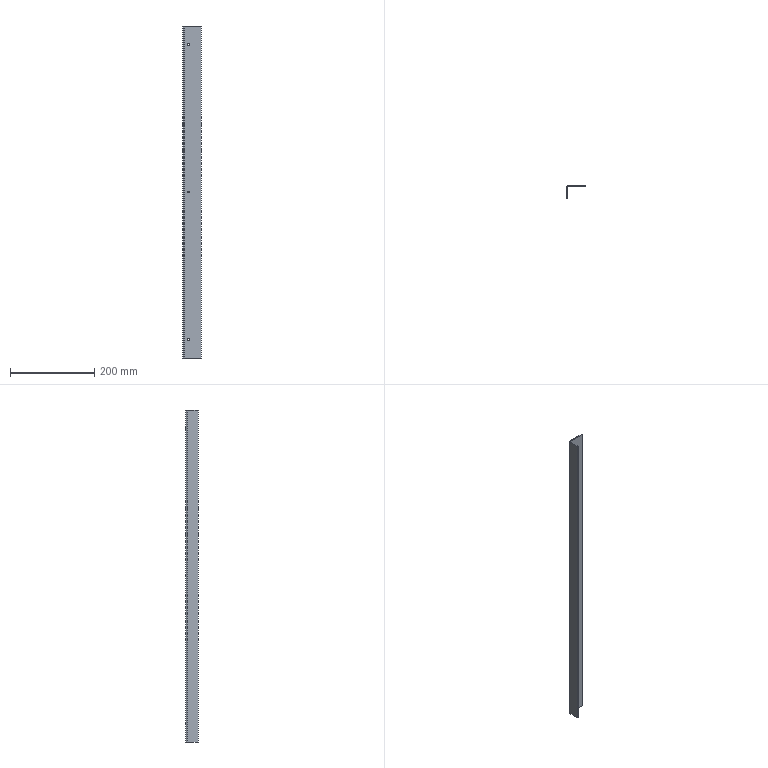Part | STEP file | SYL_0392D6J1SYL0380DJ10-1703808 | 1 solid | 20 faces | box 45 x 30 x 788 mm | volume 112936 mm3 | plane 12 | cylinder 8 | commonest cylinder face diameters 4.2 x6 4 x1 8 x1
STEP:
#1=CARTESIAN_POINT('',(-8.5,28.,-352.1));
#2=VERTEX_POINT('',#1);
#3=CARTESIAN_POINT('',(-8.5,30.,-352.1));
#4=VERTEX_POINT('',#3);
#5=CARTESIAN_POINT('',(-8.5,30.,-352.1));
#6=DIRECTION('',(0.,1.,0.));
#7=VECTOR('',#6,1000.);
#8=LINE('',#5,#7);
#9=EDGE_CURVE('',#2,#4,#8,.T.);
#10=ORIENTED_EDGE('',*,*,#9,.F.);
#11=CARTESIAN_POINT('',(-8.5,28.,-347.9));
#12=VERTEX_POINT('',#11);
#13=CARTESIAN_POINT('',(-8.5,28.,-350.));
#14=DIRECTION('',(0.,-1.,0.));
#15=DIRECTION('',(0.,0.,-1.));
#16=AXIS2_PLACEMENT_3D('',#13,#14,#15);
#17=CIRCLE('',#16,2.1);
#18=EDGE_CURVE('',#2,#12,#17,.T.);
#19=ORIENTED_EDGE('',*,*,#18,.T.);
#20=CARTESIAN_POINT('',(-8.5,30.,-347.9));
#21=VERTEX_POINT('',#20);
#22=CARTESIAN_POINT('',(-8.5,30.,-347.9));
#23=DIRECTION('',(0.,1.,0.));
#24=VECTOR('',#23,1000.);
#25=LINE('',#22,#24);
#26=EDGE_CURVE('',#12,#21,#25,.T.);
#27=ORIENTED_EDGE('',*,*,#26,.T.);
#28=CARTESIAN_POINT('',(-8.5,30.,-350.));
#29=DIRECTION('',(0.,-1.,0.));
#30=DIRECTION('',(0.,0.,-1.));
#31=AXIS2_PLACEMENT_3D('',#28,#29,#30);
#32=CIRCLE('',#31,2.1);
#33=EDGE_CURVE('',#4,#21,#32,.T.);
#34=ORIENTED_EDGE('',*,*,#33,.F.);
#35=EDGE_LOOP('',(#10,#19,#27,#34));
#36=FACE_OUTER_BOUND('',#35,.T.);
#37=CARTESIAN_POINT('',(-8.5,30.,-350.));
#38=DIRECTION('',(0.,1.,0.));
#39=DIRECTION('',(0.,0.,1.));
#40=AXIS2_PLACEMENT_3D('',#37,#38,#39);
#41=CYLINDRICAL_SURFACE('',#40,2.1);
#42=ADVANCED_FACE('',(#36),#41,.F.);
#43=CARTESIAN_POINT('',(-8.5,28.,-2.1));
#44=VERTEX_POINT('',#43);
#45=CARTESIAN_POINT('',(-8.5,30.,-2.1));
#46=VERTEX_POINT('',#45);
#47=CARTESIAN_POINT('',(-8.5,30.,-2.1));
#48=DIRECTION('',(0.,1.,0.));
#49=VECTOR('',#48,1000.);
#50=LINE('',#47,#49);
#51=EDGE_CURVE('',#44,#46,#50,.T.);
#52=ORIENTED_EDGE('',*,*,#51,.F.);
#53=CARTESIAN_POINT('',(-8.5,28.,2.1));
#54=VERTEX_POINT('',#53);
#55=CARTESIAN_POINT('',(-8.5,28.,0.));
#56=DIRECTION('',(0.,-1.,0.));
#57=DIRECTION('',(0.,0.,-1.));
#58=AXIS2_PLACEMENT_3D('',#55,#56,#57);
#59=CIRCLE('',#58,2.1);
#60=EDGE_CURVE('',#44,#54,#59,.T.);
#61=ORIENTED_EDGE('',*,*,#60,.T.);
#62=CARTESIAN_POINT('',(-8.5,30.,2.1));
#63=VERTEX_POINT('',#62);
#64=CARTESIAN_POINT('',(-8.5,30.,2.1));
#65=DIRECTION('',(0.,1.,0.));
#66=VECTOR('',#65,1000.);
#67=LINE('',#64,#66);
#68=EDGE_CURVE('',#54,#63,#67,.T.);
#69=ORIENTED_EDGE('',*,*,#68,.T.);
#70=CARTESIAN_POINT('',(-8.5,30.,0.));
#71=DIRECTION('',(0.,-1.,0.));
#72=DIRECTION('',(0.,0.,-1.));
#73=AXIS2_PLACEMENT_3D('',#70,#71,#72);
#74=CIRCLE('',#73,2.1);
#75=EDGE_CURVE('',#46,#63,#74,.T.);
#76=ORIENTED_EDGE('',*,*,#75,.F.);
#77=EDGE_LOOP('',(#52,#61,#69,#76));
#78=FACE_OUTER_BOUND('',#77,.T.);
#79=CARTESIAN_POINT('',(-8.5,30.,0.));
#80=DIRECTION('',(0.,1.,0.));
#81=DIRECTION('',(0.,0.,1.));
#82=AXIS2_PLACEMENT_3D('',#79,#80,#81);
#83=CYLINDRICAL_SURFACE('',#82,2.1);
#84=ADVANCED_FACE('',(#78),#83,.F.);
#85=CARTESIAN_POINT('',(-8.5,28.,347.9));
#86=VERTEX_POINT('',#85);
#87=CARTESIAN_POINT('',(-8.5,30.,347.9));
#88=VERTEX_POINT('',#87);
#89=CARTESIAN_POINT('',(-8.5,30.,347.9));
#90=DIRECTION('',(0.,1.,0.));
#91=VECTOR('',#90,1000.);
#92=LINE('',#89,#91);
#93=EDGE_CURVE('',#86,#88,#92,.T.);
#94=ORIENTED_EDGE('',*,*,#93,.F.);
#95=CARTESIAN_POINT('',(-8.5,28.,352.1));
#96=VERTEX_POINT('',#95);
#97=CARTESIAN_POINT('',(-8.5,28.,350.));
#98=DIRECTION('',(0.,-1.,0.));
#99=DIRECTION('',(0.,0.,-1.));
#100=AXIS2_PLACEMENT_3D('',#97,#98,#99);
#101=CIRCLE('',#100,2.1);
#102=EDGE_CURVE('',#86,#96,#101,.T.);
#103=ORIENTED_EDGE('',*,*,#102,.T.);
#104=CARTESIAN_POINT('',(-8.5,30.,352.1));
#105=VERTEX_POINT('',#104);
#106=CARTESIAN_POINT('',(-8.5,30.,352.1));
#107=DIRECTION('',(0.,1.,0.));
#108=VECTOR('',#107,1000.);
#109=LINE('',#106,#108);
#110=EDGE_CURVE('',#96,#105,#109,.T.);
#111=ORIENTED_EDGE('',*,*,#110,.T.);
#112=CARTESIAN_POINT('',(-8.5,30.,350.));
#113=DIRECTION('',(0.,-1.,0.));
#114=DIRECTION('',(0.,0.,-1.));
#115=AXIS2_PLACEMENT_3D('',#112,#113,#114);
#116=CIRCLE('',#115,2.1);
#117=EDGE_CURVE('',#88,#105,#116,.T.);
#118=ORIENTED_EDGE('',*,*,#117,.F.);
#119=EDGE_LOOP('',(#94,#103,#111,#118));
#120=FACE_OUTER_BOUND('',#119,.T.);
#121=CARTESIAN_POINT('',(-8.5,30.,350.));
#122=DIRECTION('',(0.,1.,0.));
#123=DIRECTION('',(0.,0.,1.));
#124=AXIS2_PLACEMENT_3D('',#121,#122,#123);
#125=CYLINDRICAL_SURFACE('',#124,2.1);
#126=ADVANCED_FACE('',(#120),#125,.F.);
#127=CARTESIAN_POINT('',(22.5,28.,394.));
#128=VERTEX_POINT('',#127);
#129=CARTESIAN_POINT('',(22.5,30.,394.));
#130=VERTEX_POINT('',#129);
#131=CARTESIAN_POINT('',(22.5,30.,394.));
#132=DIRECTION('',(0.,1.,0.));
#133=VECTOR('',#132,1000.);
#134=LINE('',#131,#133);
#135=EDGE_CURVE('',#128,#130,#134,.T.);
#136=ORIENTED_EDGE('',*,*,#135,.F.);
#137=CARTESIAN_POINT('',(22.5,28.,-394.));
#138=VERTEX_POINT('',#137);
#139=CARTESIAN_POINT('',(22.5,28.,-394.));
#140=DIRECTION('',(0.,0.,1.));
#141=VECTOR('',#140,1000.);
#142=LINE('',#139,#141);
#143=EDGE_CURVE('',#138,#128,#142,.T.);
#144=ORIENTED_EDGE('',*,*,#143,.F.);
#145=CARTESIAN_POINT('',(22.5,30.,-394.));
#146=VERTEX_POINT('',#145);
#147=CARTESIAN_POINT('',(22.5,30.,-394.));
#148=DIRECTION('',(0.,1.,0.));
#149=VECTOR('',#148,1000.);
#150=LINE('',#147,#149);
#151=EDGE_CURVE('',#138,#146,#150,.T.);
#152=ORIENTED_EDGE('',*,*,#151,.T.);
#153=CARTESIAN_POINT('',(22.5,30.,-394.));
#154=DIRECTION('',(0.,0.,1.));
#155=VECTOR('',#154,1000.);
#156=LINE('',#153,#155);
#157=EDGE_CURVE('',#146,#130,#156,.T.);
#158=ORIENTED_EDGE('',*,*,#157,.T.);
#159=EDGE_LOOP('',(#136,#144,#152,#158));
#160=FACE_OUTER_BOUND('',#159,.T.);
#161=CARTESIAN_POINT('',(22.5,30.,-394.));
#162=DIRECTION('',(-1.,0.,0.));
#163=DIRECTION('',(0.,0.,1.));
#164=AXIS2_PLACEMENT_3D('',#161,#162,#163);
#165=PLANE('',#164);
#166=ADVANCED_FACE('',(#160),#165,.F.);
#167=ORIENTED_EDGE('',*,*,#151,.F.);
#168=CARTESIAN_POINT('',(-18.5,28.,-394.));
#169=VERTEX_POINT('',#168);
#170=CARTESIAN_POINT('',(22.5,28.,-394.));
#171=DIRECTION('',(-1.,0.,0.));
#172=VECTOR('',#171,1000.);
#173=LINE('',#170,#172);
#174=EDGE_CURVE('',#138,#169,#173,.T.);
#175=ORIENTED_EDGE('',*,*,#174,.T.);
#176=CARTESIAN_POINT('',(-18.5,30.,-394.));
#177=VERTEX_POINT('',#176);
#178=CARTESIAN_POINT('',(-18.5,30.,-394.));
#179=DIRECTION('',(0.,1.,0.));
#180=VECTOR('',#179,1000.);
#181=LINE('',#178,#180);
#182=EDGE_CURVE('',#169,#177,#181,.T.);
#183=ORIENTED_EDGE('',*,*,#182,.T.);
#184=CARTESIAN_POINT('',(22.5,30.,-394.));
#185=DIRECTION('',(-1.,0.,0.));
#186=VECTOR('',#185,1000.);
#187=LINE('',#184,#186);
#188=EDGE_CURVE('',#146,#177,#187,.T.);
#189=ORIENTED_EDGE('',*,*,#188,.F.);
#190=EDGE_LOOP('',(#167,#175,#183,#189));
#191=FACE_OUTER_BOUND('',#190,.T.);
#192=CARTESIAN_POINT('',(22.5,30.,-394.));
#193=DIRECTION('',(0.,0.,-1.));
#194=DIRECTION('',(-1.,0.,0.));
#195=AXIS2_PLACEMENT_3D('',#192,#193,#194);
#196=PLANE('',#195);
#197=ADVANCED_FACE('',(#191),#196,.T.);
#198=ORIENTED_EDGE('',*,*,#182,.F.);
#199=CARTESIAN_POINT('',(-20.5,26.,-394.));
#200=VERTEX_POINT('',#199);
#201=CARTESIAN_POINT('',(-18.5,26.,-394.));
#202=DIRECTION('',(0.,0.,-1.));
#203=DIRECTION('',(-1.,0.,0.));
#204=AXIS2_PLACEMENT_3D('',#201,#202,#203);
#205=CIRCLE('',#204,2.);
#206=EDGE_CURVE('',#200,#169,#205,.T.);
#207=ORIENTED_EDGE('',*,*,#206,.F.);
#208=CARTESIAN_POINT('',(-22.5,26.,-394.));
#209=VERTEX_POINT('',#208);
#210=CARTESIAN_POINT('',(-22.5,26.,-394.));
#211=DIRECTION('',(-1.,0.,0.));
#212=VECTOR('',#211,1000.);
#213=LINE('',#210,#212);
#214=EDGE_CURVE('',#200,#209,#213,.T.);
#215=ORIENTED_EDGE('',*,*,#214,.T.);
#216=CARTESIAN_POINT('',(-18.5,26.,-394.));
#217=DIRECTION('',(0.,0.,-1.));
#218=DIRECTION('',(-1.,0.,0.));
#219=AXIS2_PLACEMENT_3D('',#216,#217,#218);
#220=CIRCLE('',#219,4.);
#221=EDGE_CURVE('',#209,#177,#220,.T.);
#222=ORIENTED_EDGE('',*,*,#221,.T.);
#223=EDGE_LOOP('',(#198,#207,#215,#222));
#224=FACE_OUTER_BOUND('',#223,.T.);
#225=CARTESIAN_POINT('',(-18.5,26.,-394.));
#226=DIRECTION('',(0.,0.,1.));
#227=DIRECTION('',(1.,0.,0.));
#228=AXIS2_PLACEMENT_3D('',#225,#226,#227);
#229=PLANE('',#228);
#230=ADVANCED_FACE('',(#224),#229,.F.);
#231=ORIENTED_EDGE('',*,*,#214,.F.);
#232=CARTESIAN_POINT('',(-20.5,0.,-394.));
#233=VERTEX_POINT('',#232);
#234=CARTESIAN_POINT('',(-20.5,30.,-394.));
#235=DIRECTION('',(0.,-1.,0.));
#236=VECTOR('',#235,1000.);
#237=LINE('',#234,#236);
#238=EDGE_CURVE('',#200,#233,#237,.T.);
#239=ORIENTED_EDGE('',*,*,#238,.T.);
#240=CARTESIAN_POINT('',(-22.5,0.,-394.));
#241=VERTEX_POINT('',#240);
#242=CARTESIAN_POINT('',(-22.5,0.,-394.));
#243=DIRECTION('',(-1.,0.,0.));
#244=VECTOR('',#243,1000.);
#245=LINE('',#242,#244);
#246=EDGE_CURVE('',#233,#241,#245,.T.);
#247=ORIENTED_EDGE('',*,*,#246,.T.);
#248=CARTESIAN_POINT('',(-22.5,26.,-394.));
#249=DIRECTION('',(0.,-1.,0.));
#250=VECTOR('',#249,1000.);
#251=LINE('',#248,#250);
#252=EDGE_CURVE('',#209,#241,#251,.T.);
#253=ORIENTED_EDGE('',*,*,#252,.F.);
#254=EDGE_LOOP('',(#231,#239,#247,#253));
#255=FACE_OUTER_BOUND('',#254,.T.);
#256=CARTESIAN_POINT('',(-22.5,26.,-394.));
#257=DIRECTION('',(0.,0.,-1.));
#258=DIRECTION('',(0.,-1.,0.));
#259=AXIS2_PLACEMENT_3D('',#256,#257,#258);
#260=PLANE('',#259);
#261=ADVANCED_FACE('',(#255),#260,.T.);
#262=ORIENTED_EDGE('',*,*,#246,.F.);
#263=CARTESIAN_POINT('',(-20.5,0.,394.));
#264=VERTEX_POINT('',#263);
#265=CARTESIAN_POINT('',(-20.5,0.,-394.));
#266=DIRECTION('',(0.,0.,1.));
#267=VECTOR('',#266,1000.);
#268=LINE('',#265,#267);
#269=EDGE_CURVE('',#233,#264,#268,.T.);
#270=ORIENTED_EDGE('',*,*,#269,.T.);
#271=CARTESIAN_POINT('',(-22.5,0.,394.));
#272=VERTEX_POINT('',#271);
#273=CARTESIAN_POINT('',(-22.5,0.,394.));
#274=DIRECTION('',(-1.,0.,0.));
#275=VECTOR('',#274,1000.);
#276=LINE('',#273,#275);
#277=EDGE_CURVE('',#264,#272,#276,.T.);
#278=ORIENTED_EDGE('',*,*,#277,.T.);
#279=CARTESIAN_POINT('',(-22.5,0.,-394.));
#280=DIRECTION('',(0.,0.,1.));
#281=VECTOR('',#280,1000.);
#282=LINE('',#279,#281);
#283=EDGE_CURVE('',#241,#272,#282,.T.);
#284=ORIENTED_EDGE('',*,*,#283,.F.);
#285=EDGE_LOOP('',(#262,#270,#278,#284));
#286=FACE_OUTER_BOUND('',#285,.T.);
#287=CARTESIAN_POINT('',(-22.5,0.,-394.));
#288=DIRECTION('',(0.,-1.,0.));
#289=DIRECTION('',(0.,0.,1.));
#290=AXIS2_PLACEMENT_3D('',#287,#288,#289);
#291=PLANE('',#290);
#292=ADVANCED_FACE('',(#286),#291,.T.);
#293=ORIENTED_EDGE('',*,*,#277,.F.);
#294=CARTESIAN_POINT('',(-20.5,26.,394.));
#295=VERTEX_POINT('',#294);
#296=CARTESIAN_POINT('',(-20.5,30.,394.));
#297=DIRECTION('',(0.,-1.,0.));
#298=VECTOR('',#297,1000.);
#299=LINE('',#296,#298);
#300=EDGE_CURVE('',#295,#264,#299,.T.);
#301=ORIENTED_EDGE('',*,*,#300,.F.);
#302=CARTESIAN_POINT('',(-22.5,26.,394.));
#303=VERTEX_POINT('',#302);
#304=CARTESIAN_POINT('',(-22.5,26.,394.));
#305=DIRECTION('',(-1.,0.,0.));
#306=VECTOR('',#305,1000.);
#307=LINE('',#304,#306);
#308=EDGE_CURVE('',#295,#303,#307,.T.);
#309=ORIENTED_EDGE('',*,*,#308,.T.);
#310=CARTESIAN_POINT('',(-22.5,26.,394.));
#311=DIRECTION('',(0.,-1.,0.));
#312=VECTOR('',#311,1000.);
#313=LINE('',#310,#312);
#314=EDGE_CURVE('',#303,#272,#313,.T.);
#315=ORIENTED_EDGE('',*,*,#314,.T.);
#316=EDGE_LOOP('',(#293,#301,#309,#315));
#317=FACE_OUTER_BOUND('',#316,.T.);
#318=CARTESIAN_POINT('',(-22.5,26.,394.));
#319=DIRECTION('',(0.,0.,-1.));
#320=DIRECTION('',(0.,-1.,0.));
#321=AXIS2_PLACEMENT_3D('',#318,#319,#320);
#322=PLANE('',#321);
#323=ADVANCED_FACE('',(#317),#322,.F.);
#324=ORIENTED_EDGE('',*,*,#308,.F.);
#325=CARTESIAN_POINT('',(-18.5,28.,394.));
#326=VERTEX_POINT('',#325);
#327=CARTESIAN_POINT('',(-18.5,26.,394.));
#328=DIRECTION('',(0.,0.,1.));
#329=DIRECTION('',(-1.,0.,0.));
#330=AXIS2_PLACEMENT_3D('',#327,#328,#329);
#331=CIRCLE('',#330,2.);
#332=EDGE_CURVE('',#326,#295,#331,.T.);
#333=ORIENTED_EDGE('',*,*,#332,.F.);
#334=CARTESIAN_POINT('',(-18.5,30.,394.));
#335=VERTEX_POINT('',#334);
#336=CARTESIAN_POINT('',(-18.5,30.,394.));
#337=DIRECTION('',(0.,1.,0.));
#338=VECTOR('',#337,1000.);
#339=LINE('',#336,#338);
#340=EDGE_CURVE('',#326,#335,#339,.T.);
#341=ORIENTED_EDGE('',*,*,#340,.T.);
#342=CARTESIAN_POINT('',(-18.5,26.,394.));
#343=DIRECTION('',(0.,0.,1.));
#344=DIRECTION('',(0.,1.,0.));
#345=AXIS2_PLACEMENT_3D('',#342,#343,#344);
#346=CIRCLE('',#345,4.);
#347=EDGE_CURVE('',#335,#303,#346,.T.);
#348=ORIENTED_EDGE('',*,*,#347,.T.);
#349=EDGE_LOOP('',(#324,#333,#341,#348));
#350=FACE_OUTER_BOUND('',#349,.T.);
#351=CARTESIAN_POINT('',(-18.5,26.,394.));
#352=DIRECTION('',(0.,0.,-1.));
#353=DIRECTION('',(-1.,0.,0.));
#354=AXIS2_PLACEMENT_3D('',#351,#352,#353);
#355=PLANE('',#354);
#356=ADVANCED_FACE('',(#350),#355,.F.);
#357=CARTESIAN_POINT('',(-8.5,28.,350.));
#358=DIRECTION('',(0.,-1.,0.));
#359=DIRECTION('',(0.,0.,-1.));
#360=AXIS2_PLACEMENT_3D('',#357,#358,#359);
#361=CIRCLE('',#360,2.1);
#362=EDGE_CURVE('',#96,#86,#361,.T.);
#363=ORIENTED_EDGE('',*,*,#362,.T.);
#364=ORIENTED_EDGE('',*,*,#93,.T.);
#365=CARTESIAN_POINT('',(-8.5,30.,350.));
#366=DIRECTION('',(0.,-1.,0.));
#367=DIRECTION('',(0.,0.,1.));
#368=AXIS2_PLACEMENT_3D('',#365,#366,#367);
#369=CIRCLE('',#368,2.1);
#370=EDGE_CURVE('',#105,#88,#369,.T.);
#371=ORIENTED_EDGE('',*,*,#370,.F.);
#372=ORIENTED_EDGE('',*,*,#110,.F.);
#373=EDGE_LOOP('',(#363,#364,#371,#372));
#374=FACE_OUTER_BOUND('',#373,.T.);
#375=CARTESIAN_POINT('',(-8.5,30.,350.));
#376=DIRECTION('',(0.,1.,0.));
#377=DIRECTION('',(0.,0.,1.));
#378=AXIS2_PLACEMENT_3D('',#375,#376,#377);
#379=CYLINDRICAL_SURFACE('',#378,2.1);
#380=ADVANCED_FACE('',(#374),#379,.F.);
#381=CARTESIAN_POINT('',(-8.5,28.,0.));
#382=DIRECTION('',(0.,-1.,0.));
#383=DIRECTION('',(0.,0.,-1.));
#384=AXIS2_PLACEMENT_3D('',#381,#382,#383);
#385=CIRCLE('',#384,2.1);
#386=EDGE_CURVE('',#54,#44,#385,.T.);
#387=ORIENTED_EDGE('',*,*,#386,.T.);
#388=ORIENTED_EDGE('',*,*,#51,.T.);
#389=CARTESIAN_POINT('',(-8.5,30.,0.));
#390=DIRECTION('',(0.,-1.,0.));
#391=DIRECTION('',(0.,0.,1.));
#392=AXIS2_PLACEMENT_3D('',#389,#390,#391);
#393=CIRCLE('',#392,2.1);
#394=EDGE_CURVE('',#63,#46,#393,.T.);
#395=ORIENTED_EDGE('',*,*,#394,.F.);
#396=ORIENTED_EDGE('',*,*,#68,.F.);
#397=EDGE_LOOP('',(#387,#388,#395,#396));
#398=FACE_OUTER_BOUND('',#397,.T.);
#399=CARTESIAN_POINT('',(-8.5,30.,0.));
#400=DIRECTION('',(0.,1.,0.));
#401=DIRECTION('',(0.,0.,1.));
#402=AXIS2_PLACEMENT_3D('',#399,#400,#401);
#403=CYLINDRICAL_SURFACE('',#402,2.1);
#404=ADVANCED_FACE('',(#398),#403,.F.);
#405=CARTESIAN_POINT('',(-8.5,28.,-350.));
#406=DIRECTION('',(0.,-1.,0.));
#407=DIRECTION('',(0.,0.,-1.));
#408=AXIS2_PLACEMENT_3D('',#405,#406,#407);
#409=CIRCLE('',#408,2.1);
#410=EDGE_CURVE('',#12,#2,#409,.T.);
#411=ORIENTED_EDGE('',*,*,#410,.T.);
#412=ORIENTED_EDGE('',*,*,#9,.T.);
#413=CARTESIAN_POINT('',(-8.5,30.,-350.));
#414=DIRECTION('',(0.,-1.,0.));
#415=DIRECTION('',(0.,0.,1.));
#416=AXIS2_PLACEMENT_3D('',#413,#414,#415);
#417=CIRCLE('',#416,2.1);
#418=EDGE_CURVE('',#21,#4,#417,.T.);
#419=ORIENTED_EDGE('',*,*,#418,.F.);
#420=ORIENTED_EDGE('',*,*,#26,.F.);
#421=EDGE_LOOP('',(#411,#412,#419,#420));
#422=FACE_OUTER_BOUND('',#421,.T.);
#423=CARTESIAN_POINT('',(-8.5,30.,-350.));
#424=DIRECTION('',(0.,1.,0.));
#425=DIRECTION('',(0.,0.,1.));
#426=AXIS2_PLACEMENT_3D('',#423,#424,#425);
#427=CYLINDRICAL_SURFACE('',#426,2.1);
#428=ADVANCED_FACE('',(#422),#427,.F.);
#429=CARTESIAN_POINT('',(22.5,28.,394.));
#430=DIRECTION('',(-1.,0.,0.));
#431=VECTOR('',#430,1000.);
#432=LINE('',#429,#431);
#433=EDGE_CURVE('',#128,#326,#432,.T.);
#434=ORIENTED_EDGE('',*,*,#433,.F.);
#435=ORIENTED_EDGE('',*,*,#135,.T.);
#436=CARTESIAN_POINT('',(22.5,30.,394.));
#437=DIRECTION('',(-1.,0.,0.));
#438=VECTOR('',#437,1000.);
#439=LINE('',#436,#438);
#440=EDGE_CURVE('',#130,#335,#439,.T.);
#441=ORIENTED_EDGE('',*,*,#440,.T.);
#442=ORIENTED_EDGE('',*,*,#340,.F.);
#443=EDGE_LOOP('',(#434,#435,#441,#442));
#444=FACE_OUTER_BOUND('',#443,.T.);
#445=CARTESIAN_POINT('',(22.5,30.,394.));
#446=DIRECTION('',(0.,0.,-1.));
#447=DIRECTION('',(-1.,0.,0.));
#448=AXIS2_PLACEMENT_3D('',#445,#446,#447);
#449=PLANE('',#448);
#450=ADVANCED_FACE('',(#444),#449,.F.);
#451=CARTESIAN_POINT('',(-22.5,26.,-394.));
#452=DIRECTION('',(0.,0.,1.));
#453=VECTOR('',#452,1000.);
#454=LINE('',#451,#453);
#455=EDGE_CURVE('',#209,#303,#454,.T.);
#456=ORIENTED_EDGE('',*,*,#455,.T.);
#457=ORIENTED_EDGE('',*,*,#347,.F.);
#458=CARTESIAN_POINT('',(-18.5,30.,394.));
#459=DIRECTION('',(0.,0.,-1.));
#460=VECTOR('',#459,1000.);
#461=LINE('',#458,#460);
#462=EDGE_CURVE('',#335,#177,#461,.T.);
#463=ORIENTED_EDGE('',*,*,#462,.T.);
#464=ORIENTED_EDGE('',*,*,#221,.F.);
#465=EDGE_LOOP('',(#456,#457,#463,#464));
#466=FACE_OUTER_BOUND('',#465,.T.);
#467=CARTESIAN_POINT('',(-18.5,26.,-394.));
#468=DIRECTION('',(0.,0.,-1.));
#469=DIRECTION('',(-1.,0.,0.));
#470=AXIS2_PLACEMENT_3D('',#467,#468,#469);
#471=CYLINDRICAL_SURFACE('',#470,4.);
#472=ADVANCED_FACE('',(#466),#471,.T.);
#473=ORIENTED_EDGE('',*,*,#117,.T.);
#474=ORIENTED_EDGE('',*,*,#370,.T.);
#475=EDGE_LOOP('',(#473,#474));
#476=FACE_BOUND('',#475,.T.);
#477=ORIENTED_EDGE('',*,*,#75,.T.);
#478=ORIENTED_EDGE('',*,*,#394,.T.);
#479=EDGE_LOOP('',(#477,#478));
#480=FACE_BOUND('',#479,.T.);
#481=ORIENTED_EDGE('',*,*,#33,.T.);
#482=ORIENTED_EDGE('',*,*,#418,.T.);
#483=EDGE_LOOP('',(#481,#482));
#484=FACE_BOUND('',#483,.T.);
#485=ORIENTED_EDGE('',*,*,#188,.T.);
#486=ORIENTED_EDGE('',*,*,#462,.F.);
#487=ORIENTED_EDGE('',*,*,#440,.F.);
#488=ORIENTED_EDGE('',*,*,#157,.F.);
#489=EDGE_LOOP('',(#485,#486,#487,#488));
#490=FACE_OUTER_BOUND('',#489,.T.);
#491=CARTESIAN_POINT('',(22.5,30.,-394.));
#492=DIRECTION('',(0.,1.,0.));
#493=DIRECTION('',(1.,0.,0.));
#494=AXIS2_PLACEMENT_3D('',#491,#492,#493);
#495=PLANE('',#494);
#496=ADVANCED_FACE('',(#476,#480,#484,#490),#495,.T.);
#497=ORIENTED_EDGE('',*,*,#252,.T.);
#498=ORIENTED_EDGE('',*,*,#283,.T.);
#499=ORIENTED_EDGE('',*,*,#314,.F.);
#500=ORIENTED_EDGE('',*,*,#455,.F.);
#501=EDGE_LOOP('',(#497,#498,#499,#500));
#502=FACE_OUTER_BOUND('',#501,.T.);
#503=CARTESIAN_POINT('',(-22.5,30.,-394.));
#504=DIRECTION('',(-1.,0.,0.));
#505=DIRECTION('',(0.,0.,1.));
#506=AXIS2_PLACEMENT_3D('',#503,#504,#505);
#507=PLANE('',#506);
#508=ADVANCED_FACE('',(#502),#507,.T.);
#509=CARTESIAN_POINT('',(-20.5,26.,-394.));
#510=DIRECTION('',(0.,0.,1.));
#511=VECTOR('',#510,1000.);
#512=LINE('',#509,#511);
#513=EDGE_CURVE('',#200,#295,#512,.T.);
#514=ORIENTED_EDGE('',*,*,#513,.F.);
#515=ORIENTED_EDGE('',*,*,#206,.T.);
#516=CARTESIAN_POINT('',(-18.5,28.,-394.));
#517=DIRECTION('',(0.,0.,-1.));
#518=VECTOR('',#517,1000.);
#519=LINE('',#516,#518);
#520=EDGE_CURVE('',#326,#169,#519,.T.);
#521=ORIENTED_EDGE('',*,*,#520,.F.);
#522=ORIENTED_EDGE('',*,*,#332,.T.);
#523=EDGE_LOOP('',(#514,#515,#521,#522));
#524=FACE_OUTER_BOUND('',#523,.T.);
#525=CARTESIAN_POINT('',(-18.5,26.,-394.));
#526=DIRECTION('',(0.,0.,-1.));
#527=DIRECTION('',(-1.,0.,0.));
#528=AXIS2_PLACEMENT_3D('',#525,#526,#527);
#529=CYLINDRICAL_SURFACE('',#528,2.);
#530=ADVANCED_FACE('',(#524),#529,.F.);
#531=ORIENTED_EDGE('',*,*,#102,.F.);
#532=ORIENTED_EDGE('',*,*,#362,.F.);
#533=EDGE_LOOP('',(#531,#532));
#534=FACE_BOUND('',#533,.T.);
#535=ORIENTED_EDGE('',*,*,#60,.F.);
#536=ORIENTED_EDGE('',*,*,#386,.F.);
#537=EDGE_LOOP('',(#535,#536));
#538=FACE_BOUND('',#537,.T.);
#539=ORIENTED_EDGE('',*,*,#18,.F.);
#540=ORIENTED_EDGE('',*,*,#410,.F.);
#541=EDGE_LOOP('',(#539,#540));
#542=FACE_BOUND('',#541,.T.);
#543=ORIENTED_EDGE('',*,*,#174,.F.);
#544=ORIENTED_EDGE('',*,*,#143,.T.);
#545=ORIENTED_EDGE('',*,*,#433,.T.);
#546=ORIENTED_EDGE('',*,*,#520,.T.);
#547=EDGE_LOOP('',(#543,#544,#545,#546));
#548=FACE_OUTER_BOUND('',#547,.T.);
#549=CARTESIAN_POINT('',(22.5,28.,-394.));
#550=DIRECTION('',(0.,1.,0.));
#551=DIRECTION('',(1.,0.,0.));
#552=AXIS2_PLACEMENT_3D('',#549,#550,#551);
#553=PLANE('',#552);
#554=ADVANCED_FACE('',(#534,#538,#542,#548),#553,.F.);
#555=ORIENTED_EDGE('',*,*,#238,.F.);
#556=ORIENTED_EDGE('',*,*,#513,.T.);
#557=ORIENTED_EDGE('',*,*,#300,.T.);
#558=ORIENTED_EDGE('',*,*,#269,.F.);
#559=EDGE_LOOP('',(#555,#556,#557,#558));
#560=FACE_OUTER_BOUND('',#559,.T.);
#561=CARTESIAN_POINT('',(-20.5,30.,-394.));
#562=DIRECTION('',(-1.,0.,0.));
#563=DIRECTION('',(0.,0.,1.));
#564=AXIS2_PLACEMENT_3D('',#561,#562,#563);
#565=PLANE('',#564);
#566=ADVANCED_FACE('',(#560),#565,.F.);
#567=CLOSED_SHELL('',(#42,#84,#126,#166,#197,#230,#261,#292,#323,#356,#380,#404,#428,#450,#472,#496,#508,#530,#554,#566));
#568=MANIFOLD_SOLID_BREP('',#567);
#569=CARTESIAN_POINT('',(0.,0.,0.));
#570=DIRECTION('',(0.,0.,1.));
#571=DIRECTION('',(1.,0.,0.));
#572=AXIS2_PLACEMENT_3D('',#569,#570,#571);
#573=(LENGTH_UNIT()NAMED_UNIT(*)SI_UNIT(.MILLI.,.METRE.));
#574=UNCERTAINTY_MEASURE_WITH_UNIT(LENGTH_MEASURE(0.00001),#573,'','');
#575=(NAMED_UNIT(*)PLANE_ANGLE_UNIT()SI_UNIT($,.RADIAN.));
#576=(NAMED_UNIT(*)SI_UNIT($,.STERADIAN.)SOLID_ANGLE_UNIT());
#577=(GEOMETRIC_REPRESENTATION_CONTEXT(3)GLOBAL_UNCERTAINTY_ASSIGNED_CONTEXT((#574))GLOBAL_UNIT_ASSIGNED_CONTEXT((#573,#575,#576))REPRESENTATION_CONTEXT('',''));
#578=ADVANCED_BREP_SHAPE_REPRESENTATION('',(#568,#572),#577);